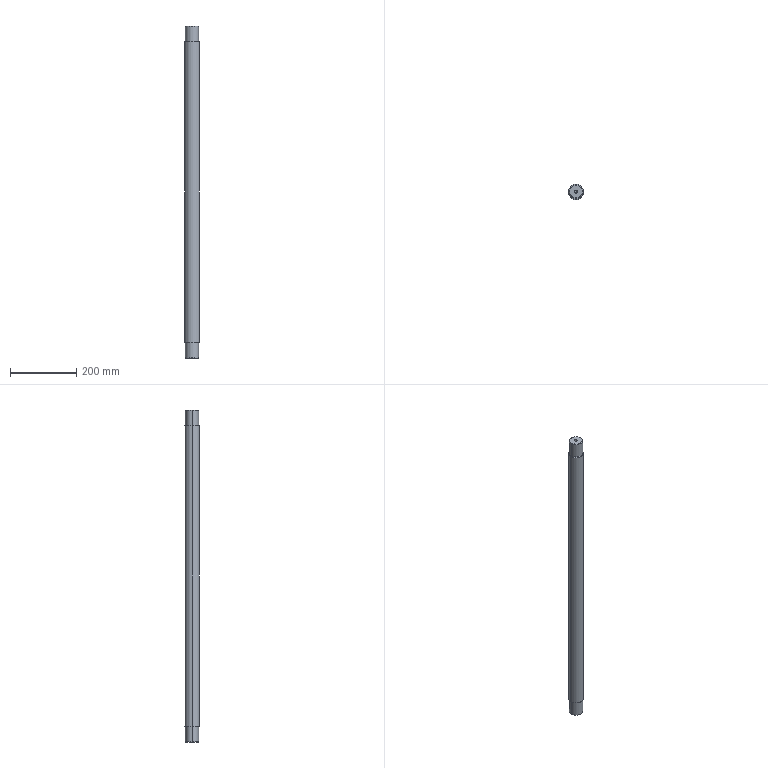Part | SolidWorks | features HoleWzd 2, ICE 2, Chamfer 1, Extrusion 1, Fillet 1 | 1 solid | 26 faces | box 45 x 45 x 1000 mm | volume 1555641 mm3 | cylinder 10 | cone 8 | torus 4 | plane 4 | commonest cylinder face diameters 8.5 x4 40 x4 45 x2
STEP:
#1=CARTESIAN_POINT('',(4.25,0.,-23.2));
#2=VERTEX_POINT('',#1);
#3=CARTESIAN_POINT('',(-4.25,0.,-23.2));
#4=VERTEX_POINT('',#3);
#5=CARTESIAN_POINT('',(0.,0.,-23.2));
#6=DIRECTION('',(0.,0.,-1.));
#7=DIRECTION('',(-1.,0.,0.));
#8=AXIS2_PLACEMENT_3D('',#5,#6,#7);
#9=CIRCLE('',#8,4.25);
#10=EDGE_CURVE('',#2,#4,#9,.T.);
#11=ORIENTED_EDGE('',*,*,#10,.F.);
#12=CARTESIAN_POINT('',(4.25,0.,-47.7));
#13=VERTEX_POINT('',#12);
#14=CARTESIAN_POINT('',(4.25,0.,-47.7));
#15=DIRECTION('',(0.,0.,-1.));
#16=VECTOR('',#15,1000.);
#17=LINE('',#14,#16);
#18=EDGE_CURVE('',#2,#13,#17,.T.);
#19=ORIENTED_EDGE('',*,*,#18,.T.);
#20=CARTESIAN_POINT('',(-4.25,0.,-47.7));
#21=VERTEX_POINT('',#20);
#22=CARTESIAN_POINT('',(0.,0.,-47.7));
#23=DIRECTION('',(0.,0.,-1.));
#24=DIRECTION('',(-1.,0.,0.));
#25=AXIS2_PLACEMENT_3D('',#22,#23,#24);
#26=CIRCLE('',#25,4.25);
#27=EDGE_CURVE('',#13,#21,#26,.T.);
#28=ORIENTED_EDGE('',*,*,#27,.T.);
#29=CARTESIAN_POINT('',(-4.25,0.,-47.7));
#30=DIRECTION('',(0.,0.,-1.));
#31=VECTOR('',#30,1000.);
#32=LINE('',#29,#31);
#33=EDGE_CURVE('',#4,#21,#32,.T.);
#34=ORIENTED_EDGE('',*,*,#33,.F.);
#35=EDGE_LOOP('',(#11,#19,#28,#34));
#36=FACE_OUTER_BOUND('',#35,.T.);
#37=CARTESIAN_POINT('',(0.,0.,-47.7));
#38=DIRECTION('',(0.,0.,-1.));
#39=DIRECTION('',(-1.,0.,0.));
#40=AXIS2_PLACEMENT_3D('',#37,#38,#39);
#41=CYLINDRICAL_SURFACE('',#40,4.25);
#42=ADVANCED_FACE('',(#36),#41,.F.);
#43=CARTESIAN_POINT('',(0.,0.,-20.646));
#44=VERTEX_POINT('',#43);
#45=CARTESIAN_POINT('',(-4.25,0.,-23.2));
#46=DIRECTION('',(-0.8572,0.,-0.515));
#47=VECTOR('',#46,1000.);
#48=LINE('',#45,#47);
#49=EDGE_CURVE('',#44,#4,#48,.T.);
#50=ORIENTED_EDGE('',*,*,#49,.F.);
#51=CARTESIAN_POINT('',(4.25,0.,-23.2));
#52=DIRECTION('',(0.8572,0.,-0.515));
#53=VECTOR('',#52,1000.);
#54=LINE('',#51,#53);
#55=EDGE_CURVE('',#44,#2,#54,.T.);
#56=ORIENTED_EDGE('',*,*,#55,.T.);
#57=ORIENTED_EDGE('',*,*,#10,.T.);
#58=EDGE_LOOP('',(#50,#56,#57));
#59=FACE_OUTER_BOUND('',#58,.T.);
#60=CARTESIAN_POINT('',(0.,0.,-23.2));
#61=DIRECTION('',(0.,0.,-1.));
#62=DIRECTION('',(-1.,0.,0.));
#63=AXIS2_PLACEMENT_3D('',#60,#61,#62);
#64=CONICAL_SURFACE('',#63,4.25,1.03);
#65=ADVANCED_FACE('',(#59),#64,.F.);
#66=CARTESIAN_POINT('',(-4.25,0.,927.8));
#67=VERTEX_POINT('',#66);
#68=CARTESIAN_POINT('',(4.25,0.,927.8));
#69=VERTEX_POINT('',#68);
#70=CARTESIAN_POINT('',(0.,0.,927.8));
#71=DIRECTION('',(0.,0.,1.));
#72=DIRECTION('',(1.,0.,0.));
#73=AXIS2_PLACEMENT_3D('',#70,#71,#72);
#74=CIRCLE('',#73,4.25);
#75=EDGE_CURVE('',#67,#69,#74,.T.);
#76=ORIENTED_EDGE('',*,*,#75,.F.);
#77=CARTESIAN_POINT('',(-4.25,0.,952.3));
#78=VERTEX_POINT('',#77);
#79=CARTESIAN_POINT('',(-4.25,0.,952.3));
#80=DIRECTION('',(0.,0.,1.));
#81=VECTOR('',#80,1000.);
#82=LINE('',#79,#81);
#83=EDGE_CURVE('',#67,#78,#82,.T.);
#84=ORIENTED_EDGE('',*,*,#83,.T.);
#85=CARTESIAN_POINT('',(4.25,0.,952.3));
#86=VERTEX_POINT('',#85);
#87=CARTESIAN_POINT('',(0.,0.,952.3));
#88=DIRECTION('',(0.,0.,1.));
#89=DIRECTION('',(1.,0.,0.));
#90=AXIS2_PLACEMENT_3D('',#87,#88,#89);
#91=CIRCLE('',#90,4.25);
#92=EDGE_CURVE('',#78,#86,#91,.T.);
#93=ORIENTED_EDGE('',*,*,#92,.T.);
#94=CARTESIAN_POINT('',(4.25,0.,952.3));
#95=DIRECTION('',(0.,0.,1.));
#96=VECTOR('',#95,1000.);
#97=LINE('',#94,#96);
#98=EDGE_CURVE('',#69,#86,#97,.T.);
#99=ORIENTED_EDGE('',*,*,#98,.F.);
#100=EDGE_LOOP('',(#76,#84,#93,#99));
#101=FACE_OUTER_BOUND('',#100,.T.);
#102=CARTESIAN_POINT('',(0.,0.,952.3));
#103=DIRECTION('',(0.,0.,1.));
#104=DIRECTION('',(1.,0.,0.));
#105=AXIS2_PLACEMENT_3D('',#102,#103,#104);
#106=CYLINDRICAL_SURFACE('',#105,4.25);
#107=ADVANCED_FACE('',(#101),#106,.F.);
#108=CARTESIAN_POINT('',(0.,0.,925.246));
#109=VERTEX_POINT('',#108);
#110=CARTESIAN_POINT('',(4.25,0.,927.8));
#111=DIRECTION('',(0.8572,0.,0.515));
#112=VECTOR('',#111,1000.);
#113=LINE('',#110,#112);
#114=EDGE_CURVE('',#109,#69,#113,.T.);
#115=ORIENTED_EDGE('',*,*,#114,.F.);
#116=CARTESIAN_POINT('',(-4.25,0.,927.8));
#117=DIRECTION('',(-0.8572,0.,0.515));
#118=VECTOR('',#117,1000.);
#119=LINE('',#116,#118);
#120=EDGE_CURVE('',#109,#67,#119,.T.);
#121=ORIENTED_EDGE('',*,*,#120,.T.);
#122=ORIENTED_EDGE('',*,*,#75,.T.);
#123=EDGE_LOOP('',(#115,#121,#122));
#124=FACE_OUTER_BOUND('',#123,.T.);
#125=CARTESIAN_POINT('',(0.,0.,927.8));
#126=DIRECTION('',(0.,0.,1.));
#127=DIRECTION('',(1.,0.,0.));
#128=AXIS2_PLACEMENT_3D('',#125,#126,#127);
#129=CONICAL_SURFACE('',#128,4.25,1.03);
#130=ADVANCED_FACE('',(#124),#129,.F.);
#131=CARTESIAN_POINT('',(-19.,0.,-47.7));
#132=VERTEX_POINT('',#131);
#133=CARTESIAN_POINT('',(19.,0.,-47.7));
#134=VERTEX_POINT('',#133);
#135=CARTESIAN_POINT('',(0.,0.,-47.7));
#136=DIRECTION('',(0.,0.,-1.));
#137=DIRECTION('',(-1.,0.,0.));
#138=AXIS2_PLACEMENT_3D('',#135,#136,#137);
#139=CIRCLE('',#138,19.);
#140=EDGE_CURVE('',#132,#134,#139,.T.);
#141=ORIENTED_EDGE('',*,*,#140,.F.);
#142=CARTESIAN_POINT('',(-20.,0.,-46.7));
#143=VERTEX_POINT('',#142);
#144=CARTESIAN_POINT('',(-19.,0.,-47.7));
#145=DIRECTION('',(-0.7071,0.,0.7071));
#146=VECTOR('',#145,1000.);
#147=LINE('',#144,#146);
#148=EDGE_CURVE('',#132,#143,#147,.T.);
#149=ORIENTED_EDGE('',*,*,#148,.T.);
#150=CARTESIAN_POINT('',(20.,0.,-46.7));
#151=VERTEX_POINT('',#150);
#152=CARTESIAN_POINT('',(0.,0.,-46.7));
#153=DIRECTION('',(0.,0.,1.));
#154=DIRECTION('',(-1.,0.,0.));
#155=AXIS2_PLACEMENT_3D('',#152,#153,#154);
#156=CIRCLE('',#155,20.);
#157=EDGE_CURVE('',#151,#143,#156,.T.);
#158=ORIENTED_EDGE('',*,*,#157,.F.);
#159=CARTESIAN_POINT('',(19.,0.,-47.7));
#160=DIRECTION('',(0.7071,0.,0.7071));
#161=VECTOR('',#160,1000.);
#162=LINE('',#159,#161);
#163=EDGE_CURVE('',#134,#151,#162,.T.);
#164=ORIENTED_EDGE('',*,*,#163,.F.);
#165=EDGE_LOOP('',(#141,#149,#158,#164));
#166=FACE_OUTER_BOUND('',#165,.T.);
#167=CARTESIAN_POINT('',(0.,0.,-47.7));
#168=DIRECTION('',(0.,0.,1.));
#169=DIRECTION('',(1.,0.,0.));
#170=AXIS2_PLACEMENT_3D('',#167,#168,#169);
#171=CONICAL_SURFACE('',#170,19.,0.7854);
#172=ADVANCED_FACE('',(#166),#171,.T.);
#173=CARTESIAN_POINT('',(19.,0.,952.3));
#174=VERTEX_POINT('',#173);
#175=CARTESIAN_POINT('',(-19.,0.,952.3));
#176=VERTEX_POINT('',#175);
#177=CARTESIAN_POINT('',(0.,0.,952.3));
#178=DIRECTION('',(0.,0.,1.));
#179=DIRECTION('',(1.,0.,0.));
#180=AXIS2_PLACEMENT_3D('',#177,#178,#179);
#181=CIRCLE('',#180,19.);
#182=EDGE_CURVE('',#174,#176,#181,.T.);
#183=ORIENTED_EDGE('',*,*,#182,.F.);
#184=CARTESIAN_POINT('',(20.,0.,951.3));
#185=VERTEX_POINT('',#184);
#186=CARTESIAN_POINT('',(19.,0.,952.3));
#187=DIRECTION('',(0.7071,0.,-0.7071));
#188=VECTOR('',#187,1000.);
#189=LINE('',#186,#188);
#190=EDGE_CURVE('',#174,#185,#189,.T.);
#191=ORIENTED_EDGE('',*,*,#190,.T.);
#192=CARTESIAN_POINT('',(-20.,0.,951.3));
#193=VERTEX_POINT('',#192);
#194=CARTESIAN_POINT('',(0.,0.,951.3));
#195=DIRECTION('',(0.,0.,-1.));
#196=DIRECTION('',(1.,0.,0.));
#197=AXIS2_PLACEMENT_3D('',#194,#195,#196);
#198=CIRCLE('',#197,20.);
#199=EDGE_CURVE('',#193,#185,#198,.T.);
#200=ORIENTED_EDGE('',*,*,#199,.F.);
#201=CARTESIAN_POINT('',(-19.,0.,952.3));
#202=DIRECTION('',(-0.7071,0.,-0.7071));
#203=VECTOR('',#202,1000.);
#204=LINE('',#201,#203);
#205=EDGE_CURVE('',#176,#193,#204,.T.);
#206=ORIENTED_EDGE('',*,*,#205,.F.);
#207=EDGE_LOOP('',(#183,#191,#200,#206));
#208=FACE_OUTER_BOUND('',#207,.T.);
#209=CARTESIAN_POINT('',(0.,0.,952.3));
#210=DIRECTION('',(0.,0.,-1.));
#211=DIRECTION('',(-1.,0.,0.));
#212=AXIS2_PLACEMENT_3D('',#209,#210,#211);
#213=CONICAL_SURFACE('',#212,19.,0.7854);
#214=ADVANCED_FACE('',(#208),#213,.T.);
#215=CARTESIAN_POINT('',(-20.,0.,905.6));
#216=VERTEX_POINT('',#215);
#217=CARTESIAN_POINT('',(20.,0.,905.6));
#218=VERTEX_POINT('',#217);
#219=CARTESIAN_POINT('',(0.,0.,905.6));
#220=DIRECTION('',(0.,0.,1.));
#221=DIRECTION('',(1.,0.,0.));
#222=AXIS2_PLACEMENT_3D('',#219,#220,#221);
#223=CIRCLE('',#222,20.);
#224=EDGE_CURVE('',#216,#218,#223,.T.);
#225=ORIENTED_EDGE('',*,*,#224,.F.);
#226=CARTESIAN_POINT('',(-21.,0.,904.6));
#227=VERTEX_POINT('',#226);
#228=CARTESIAN_POINT('',(-21.,0.,905.6));
#229=DIRECTION('',(0.,1.,0.));
#230=DIRECTION('',(-1.,0.,0.));
#231=AXIS2_PLACEMENT_3D('',#228,#229,#230);
#232=CIRCLE('',#231,1.);
#233=EDGE_CURVE('',#216,#227,#232,.T.);
#234=ORIENTED_EDGE('',*,*,#233,.T.);
#235=CARTESIAN_POINT('',(21.,0.,904.6));
#236=VERTEX_POINT('',#235);
#237=CARTESIAN_POINT('',(0.,0.,904.6));
#238=DIRECTION('',(0.,0.,-1.));
#239=DIRECTION('',(1.,0.,0.));
#240=AXIS2_PLACEMENT_3D('',#237,#238,#239);
#241=CIRCLE('',#240,21.);
#242=EDGE_CURVE('',#236,#227,#241,.T.);
#243=ORIENTED_EDGE('',*,*,#242,.F.);
#244=CARTESIAN_POINT('',(21.,0.,905.6));
#245=DIRECTION('',(0.,-1.,0.));
#246=DIRECTION('',(0.,0.,-1.));
#247=AXIS2_PLACEMENT_3D('',#244,#245,#246);
#248=CIRCLE('',#247,1.);
#249=EDGE_CURVE('',#218,#236,#248,.T.);
#250=ORIENTED_EDGE('',*,*,#249,.F.);
#251=EDGE_LOOP('',(#225,#234,#243,#250));
#252=FACE_OUTER_BOUND('',#251,.T.);
#253=CARTESIAN_POINT('',(0.,0.,905.6));
#254=DIRECTION('',(0.,0.,1.));
#255=DIRECTION('',(1.,0.,0.));
#256=AXIS2_PLACEMENT_3D('',#253,#254,#255);
#257=TOROIDAL_SURFACE('',#256,21.,1.);
#258=ADVANCED_FACE('',(#252),#257,.F.);
#259=CARTESIAN_POINT('',(-21.,0.,0.));
#260=VERTEX_POINT('',#259);
#261=CARTESIAN_POINT('',(21.,0.,0.));
#262=VERTEX_POINT('',#261);
#263=CARTESIAN_POINT('',(0.,0.,0.));
#264=DIRECTION('',(0.,0.,1.));
#265=DIRECTION('',(1.,0.,0.));
#266=AXIS2_PLACEMENT_3D('',#263,#264,#265);
#267=CIRCLE('',#266,21.);
#268=EDGE_CURVE('',#260,#262,#267,.T.);
#269=ORIENTED_EDGE('',*,*,#268,.F.);
#270=CARTESIAN_POINT('',(-20.,0.,-1.));
#271=VERTEX_POINT('',#270);
#272=CARTESIAN_POINT('',(-21.,0.,-1.));
#273=DIRECTION('',(0.,1.,0.));
#274=DIRECTION('',(-1.,0.,0.));
#275=AXIS2_PLACEMENT_3D('',#272,#273,#274);
#276=CIRCLE('',#275,1.);
#277=EDGE_CURVE('',#260,#271,#276,.T.);
#278=ORIENTED_EDGE('',*,*,#277,.T.);
#279=CARTESIAN_POINT('',(20.,0.,-1.));
#280=VERTEX_POINT('',#279);
#281=CARTESIAN_POINT('',(0.,0.,-1.));
#282=DIRECTION('',(0.,0.,-1.));
#283=DIRECTION('',(1.,0.,0.));
#284=AXIS2_PLACEMENT_3D('',#281,#282,#283);
#285=CIRCLE('',#284,20.);
#286=EDGE_CURVE('',#280,#271,#285,.T.);
#287=ORIENTED_EDGE('',*,*,#286,.F.);
#288=CARTESIAN_POINT('',(21.,0.,-1.));
#289=DIRECTION('',(0.,-1.,0.));
#290=DIRECTION('',(0.,0.,-1.));
#291=AXIS2_PLACEMENT_3D('',#288,#289,#290);
#292=CIRCLE('',#291,1.);
#293=EDGE_CURVE('',#262,#280,#292,.T.);
#294=ORIENTED_EDGE('',*,*,#293,.F.);
#295=EDGE_LOOP('',(#269,#278,#287,#294));
#296=FACE_OUTER_BOUND('',#295,.T.);
#297=CARTESIAN_POINT('',(0.,0.,-1.));
#298=DIRECTION('',(0.,0.,1.));
#299=DIRECTION('',(1.,0.,0.));
#300=AXIS2_PLACEMENT_3D('',#297,#298,#299);
#301=TOROIDAL_SURFACE('',#300,21.,1.);
#302=ADVANCED_FACE('',(#296),#301,.F.);
#303=ORIENTED_EDGE('',*,*,#157,.T.);
#304=CARTESIAN_POINT('',(-20.,0.,-47.7));
#305=DIRECTION('',(0.,0.,1.));
#306=VECTOR('',#305,1000.);
#307=LINE('',#304,#306);
#308=EDGE_CURVE('',#143,#271,#307,.T.);
#309=ORIENTED_EDGE('',*,*,#308,.T.);
#310=CARTESIAN_POINT('',(0.,0.,-1.));
#311=DIRECTION('',(0.,0.,-1.));
#312=DIRECTION('',(1.,0.,0.));
#313=AXIS2_PLACEMENT_3D('',#310,#311,#312);
#314=CIRCLE('',#313,20.);
#315=EDGE_CURVE('',#271,#280,#314,.T.);
#316=ORIENTED_EDGE('',*,*,#315,.T.);
#317=CARTESIAN_POINT('',(20.,0.,-47.7));
#318=DIRECTION('',(0.,0.,1.));
#319=VECTOR('',#318,1000.);
#320=LINE('',#317,#319);
#321=EDGE_CURVE('',#151,#280,#320,.T.);
#322=ORIENTED_EDGE('',*,*,#321,.F.);
#323=EDGE_LOOP('',(#303,#309,#316,#322));
#324=FACE_OUTER_BOUND('',#323,.T.);
#325=CARTESIAN_POINT('',(0.,0.,-47.7));
#326=DIRECTION('',(0.,0.,1.));
#327=DIRECTION('',(1.,0.,0.));
#328=AXIS2_PLACEMENT_3D('',#325,#326,#327);
#329=CYLINDRICAL_SURFACE('',#328,20.);
#330=ADVANCED_FACE('',(#324),#329,.T.);
#331=ORIENTED_EDGE('',*,*,#199,.T.);
#332=CARTESIAN_POINT('',(20.,0.,952.3));
#333=DIRECTION('',(0.,0.,-1.));
#334=VECTOR('',#333,1000.);
#335=LINE('',#332,#334);
#336=EDGE_CURVE('',#185,#218,#335,.T.);
#337=ORIENTED_EDGE('',*,*,#336,.T.);
#338=CARTESIAN_POINT('',(0.,0.,905.6));
#339=DIRECTION('',(0.,0.,1.));
#340=DIRECTION('',(1.,0.,0.));
#341=AXIS2_PLACEMENT_3D('',#338,#339,#340);
#342=CIRCLE('',#341,20.);
#343=EDGE_CURVE('',#218,#216,#342,.T.);
#344=ORIENTED_EDGE('',*,*,#343,.T.);
#345=CARTESIAN_POINT('',(-20.,0.,952.3));
#346=DIRECTION('',(0.,0.,-1.));
#347=VECTOR('',#346,1000.);
#348=LINE('',#345,#347);
#349=EDGE_CURVE('',#193,#216,#348,.T.);
#350=ORIENTED_EDGE('',*,*,#349,.F.);
#351=EDGE_LOOP('',(#331,#337,#344,#350));
#352=FACE_OUTER_BOUND('',#351,.T.);
#353=CARTESIAN_POINT('',(0.,0.,952.3));
#354=DIRECTION('',(0.,0.,-1.));
#355=DIRECTION('',(-1.,0.,0.));
#356=AXIS2_PLACEMENT_3D('',#353,#354,#355);
#357=CYLINDRICAL_SURFACE('',#356,20.);
#358=ADVANCED_FACE('',(#352),#357,.T.);
#359=CARTESIAN_POINT('',(22.5,0.,904.6));
#360=VERTEX_POINT('',#359);
#361=CARTESIAN_POINT('',(-22.5,0.,904.6));
#362=VERTEX_POINT('',#361);
#363=CARTESIAN_POINT('',(0.,0.,904.6));
#364=DIRECTION('',(0.,0.,1.));
#365=DIRECTION('',(1.,0.,0.));
#366=AXIS2_PLACEMENT_3D('',#363,#364,#365);
#367=CIRCLE('',#366,22.5);
#368=EDGE_CURVE('',#360,#362,#367,.T.);
#369=ORIENTED_EDGE('',*,*,#368,.F.);
#370=CARTESIAN_POINT('',(22.5,0.,0.));
#371=VERTEX_POINT('',#370);
#372=CARTESIAN_POINT('',(22.5,0.,904.6));
#373=DIRECTION('',(0.,0.,-1.));
#374=VECTOR('',#373,1000.);
#375=LINE('',#372,#374);
#376=EDGE_CURVE('',#360,#371,#375,.T.);
#377=ORIENTED_EDGE('',*,*,#376,.T.);
#378=CARTESIAN_POINT('',(-22.5,0.,0.));
#379=VERTEX_POINT('',#378);
#380=CARTESIAN_POINT('',(0.,0.,0.));
#381=DIRECTION('',(0.,0.,1.));
#382=DIRECTION('',(1.,0.,0.));
#383=AXIS2_PLACEMENT_3D('',#380,#381,#382);
#384=CIRCLE('',#383,22.5);
#385=EDGE_CURVE('',#371,#379,#384,.T.);
#386=ORIENTED_EDGE('',*,*,#385,.T.);
#387=CARTESIAN_POINT('',(-22.5,0.,904.6));
#388=DIRECTION('',(0.,0.,-1.));
#389=VECTOR('',#388,1000.);
#390=LINE('',#387,#389);
#391=EDGE_CURVE('',#362,#379,#390,.T.);
#392=ORIENTED_EDGE('',*,*,#391,.F.);
#393=EDGE_LOOP('',(#369,#377,#386,#392));
#394=FACE_OUTER_BOUND('',#393,.T.);
#395=CARTESIAN_POINT('',(0.,0.,904.6));
#396=DIRECTION('',(0.,0.,-1.));
#397=DIRECTION('',(-1.,0.,0.));
#398=AXIS2_PLACEMENT_3D('',#395,#396,#397);
#399=CYLINDRICAL_SURFACE('',#398,22.5);
#400=ADVANCED_FACE('',(#394),#399,.T.);
#401=ORIENTED_EDGE('',*,*,#376,.F.);
#402=CARTESIAN_POINT('',(0.,0.,904.6));
#403=DIRECTION('',(0.,0.,1.));
#404=DIRECTION('',(1.,0.,0.));
#405=AXIS2_PLACEMENT_3D('',#402,#403,#404);
#406=CIRCLE('',#405,22.5);
#407=EDGE_CURVE('',#362,#360,#406,.T.);
#408=ORIENTED_EDGE('',*,*,#407,.F.);
#409=ORIENTED_EDGE('',*,*,#391,.T.);
#410=CARTESIAN_POINT('',(0.,0.,0.));
#411=DIRECTION('',(0.,0.,1.));
#412=DIRECTION('',(1.,0.,0.));
#413=AXIS2_PLACEMENT_3D('',#410,#411,#412);
#414=CIRCLE('',#413,22.5);
#415=EDGE_CURVE('',#379,#371,#414,.T.);
#416=ORIENTED_EDGE('',*,*,#415,.T.);
#417=EDGE_LOOP('',(#401,#408,#409,#416));
#418=FACE_OUTER_BOUND('',#417,.T.);
#419=CARTESIAN_POINT('',(0.,0.,904.6));
#420=DIRECTION('',(0.,0.,-1.));
#421=DIRECTION('',(-1.,0.,0.));
#422=AXIS2_PLACEMENT_3D('',#419,#420,#421);
#423=CYLINDRICAL_SURFACE('',#422,22.5);
#424=ADVANCED_FACE('',(#418),#423,.T.);
#425=ORIENTED_EDGE('',*,*,#242,.T.);
#426=CARTESIAN_POINT('',(0.,0.,904.6));
#427=DIRECTION('',(0.,0.,-1.));
#428=DIRECTION('',(1.,0.,0.));
#429=AXIS2_PLACEMENT_3D('',#426,#427,#428);
#430=CIRCLE('',#429,21.);
#431=EDGE_CURVE('',#227,#236,#430,.T.);
#432=ORIENTED_EDGE('',*,*,#431,.T.);
#433=EDGE_LOOP('',(#425,#432));
#434=FACE_BOUND('',#433,.T.);
#435=ORIENTED_EDGE('',*,*,#407,.T.);
#436=ORIENTED_EDGE('',*,*,#368,.T.);
#437=EDGE_LOOP('',(#435,#436));
#438=FACE_OUTER_BOUND('',#437,.T.);
#439=CARTESIAN_POINT('',(0.,0.,904.6));
#440=DIRECTION('',(0.,0.,1.));
#441=DIRECTION('',(1.,0.,0.));
#442=AXIS2_PLACEMENT_3D('',#439,#440,#441);
#443=PLANE('',#442);
#444=ADVANCED_FACE('',(#434,#438),#443,.T.);
#445=CARTESIAN_POINT('',(0.,0.,0.));
#446=DIRECTION('',(0.,0.,1.));
#447=DIRECTION('',(1.,0.,0.));
#448=AXIS2_PLACEMENT_3D('',#445,#446,#447);
#449=CIRCLE('',#448,21.);
#450=EDGE_CURVE('',#262,#260,#449,.T.);
#451=ORIENTED_EDGE('',*,*,#450,.T.);
#452=ORIENTED_EDGE('',*,*,#268,.T.);
#453=EDGE_LOOP('',(#451,#452));
#454=FACE_BOUND('',#453,.T.);
#455=ORIENTED_EDGE('',*,*,#415,.F.);
#456=ORIENTED_EDGE('',*,*,#385,.F.);
#457=EDGE_LOOP('',(#455,#456));
#458=FACE_OUTER_BOUND('',#457,.T.);
#459=CARTESIAN_POINT('',(0.,0.,0.));
#460=DIRECTION('',(0.,0.,1.));
#461=DIRECTION('',(1.,0.,0.));
#462=AXIS2_PLACEMENT_3D('',#459,#460,#461);
#463=PLANE('',#462);
#464=ADVANCED_FACE('',(#454,#458),#463,.F.);
#465=ORIENTED_EDGE('',*,*,#336,.F.);
#466=CARTESIAN_POINT('',(0.,0.,951.3));
#467=DIRECTION('',(0.,0.,-1.));
#468=DIRECTION('',(1.,0.,0.));
#469=AXIS2_PLACEMENT_3D('',#466,#467,#468);
#470=CIRCLE('',#469,20.);
#471=EDGE_CURVE('',#185,#193,#470,.T.);
#472=ORIENTED_EDGE('',*,*,#471,.T.);
#473=ORIENTED_EDGE('',*,*,#349,.T.);
#474=ORIENTED_EDGE('',*,*,#224,.T.);
#475=EDGE_LOOP('',(#465,#472,#473,#474));
#476=FACE_OUTER_BOUND('',#475,.T.);
#477=CARTESIAN_POINT('',(0.,0.,952.3));
#478=DIRECTION('',(0.,0.,-1.));
#479=DIRECTION('',(-1.,0.,0.));
#480=AXIS2_PLACEMENT_3D('',#477,#478,#479);
#481=CYLINDRICAL_SURFACE('',#480,20.);
#482=ADVANCED_FACE('',(#476),#481,.T.);
#483=CARTESIAN_POINT('',(0.,0.,952.3));
#484=DIRECTION('',(0.,0.,1.));
#485=DIRECTION('',(1.,0.,0.));
#486=AXIS2_PLACEMENT_3D('',#483,#484,#485);
#487=CIRCLE('',#486,4.25);
#488=EDGE_CURVE('',#86,#78,#487,.T.);
#489=ORIENTED_EDGE('',*,*,#488,.F.);
#490=ORIENTED_EDGE('',*,*,#92,.F.);
#491=EDGE_LOOP('',(#489,#490));
#492=FACE_BOUND('',#491,.T.);
#493=CARTESIAN_POINT('',(0.,0.,952.3));
#494=DIRECTION('',(0.,0.,1.));
#495=DIRECTION('',(1.,0.,0.));
#496=AXIS2_PLACEMENT_3D('',#493,#494,#495);
#497=CIRCLE('',#496,19.);
#498=EDGE_CURVE('',#176,#174,#497,.T.);
#499=ORIENTED_EDGE('',*,*,#498,.T.);
#500=ORIENTED_EDGE('',*,*,#182,.T.);
#501=EDGE_LOOP('',(#499,#500));
#502=FACE_OUTER_BOUND('',#501,.T.);
#503=CARTESIAN_POINT('',(0.,0.,952.3));
#504=DIRECTION('',(0.,0.,1.));
#505=DIRECTION('',(1.,0.,0.));
#506=AXIS2_PLACEMENT_3D('',#503,#504,#505);
#507=PLANE('',#506);
#508=ADVANCED_FACE('',(#492,#502),#507,.T.);
#509=ORIENTED_EDGE('',*,*,#308,.F.);
#510=CARTESIAN_POINT('',(0.,0.,-46.7));
#511=DIRECTION('',(0.,0.,1.));
#512=DIRECTION('',(-1.,0.,0.));
#513=AXIS2_PLACEMENT_3D('',#510,#511,#512);
#514=CIRCLE('',#513,20.);
#515=EDGE_CURVE('',#143,#151,#514,.T.);
#516=ORIENTED_EDGE('',*,*,#515,.T.);
#517=ORIENTED_EDGE('',*,*,#321,.T.);
#518=ORIENTED_EDGE('',*,*,#286,.T.);
#519=EDGE_LOOP('',(#509,#516,#517,#518));
#520=FACE_OUTER_BOUND('',#519,.T.);
#521=CARTESIAN_POINT('',(0.,0.,-47.7));
#522=DIRECTION('',(0.,0.,1.));
#523=DIRECTION('',(1.,0.,0.));
#524=AXIS2_PLACEMENT_3D('',#521,#522,#523);
#525=CYLINDRICAL_SURFACE('',#524,20.);
#526=ADVANCED_FACE('',(#520),#525,.T.);
#527=CARTESIAN_POINT('',(0.,0.,-47.7));
#528=DIRECTION('',(0.,0.,-1.));
#529=DIRECTION('',(-1.,0.,0.));
#530=AXIS2_PLACEMENT_3D('',#527,#528,#529);
#531=CIRCLE('',#530,4.25);
#532=EDGE_CURVE('',#21,#13,#531,.T.);
#533=ORIENTED_EDGE('',*,*,#532,.F.);
#534=ORIENTED_EDGE('',*,*,#27,.F.);
#535=EDGE_LOOP('',(#533,#534));
#536=FACE_BOUND('',#535,.T.);
#537=CARTESIAN_POINT('',(0.,0.,-47.7));
#538=DIRECTION('',(0.,0.,-1.));
#539=DIRECTION('',(-1.,0.,0.));
#540=AXIS2_PLACEMENT_3D('',#537,#538,#539);
#541=CIRCLE('',#540,19.);
#542=EDGE_CURVE('',#134,#132,#541,.T.);
#543=ORIENTED_EDGE('',*,*,#542,.T.);
#544=ORIENTED_EDGE('',*,*,#140,.T.);
#545=EDGE_LOOP('',(#543,#544));
#546=FACE_OUTER_BOUND('',#545,.T.);
#547=CARTESIAN_POINT('',(0.,0.,-47.7));
#548=DIRECTION('',(0.,0.,-1.));
#549=DIRECTION('',(-1.,0.,0.));
#550=AXIS2_PLACEMENT_3D('',#547,#548,#549);
#551=PLANE('',#550);
#552=ADVANCED_FACE('',(#536,#546),#551,.T.);
#553=ORIENTED_EDGE('',*,*,#277,.F.);
#554=ORIENTED_EDGE('',*,*,#450,.F.);
#555=ORIENTED_EDGE('',*,*,#293,.T.);
#556=ORIENTED_EDGE('',*,*,#315,.F.);
#557=EDGE_LOOP('',(#553,#554,#555,#556));
#558=FACE_OUTER_BOUND('',#557,.T.);
#559=CARTESIAN_POINT('',(0.,0.,-1.));
#560=DIRECTION('',(0.,0.,1.));
#561=DIRECTION('',(1.,0.,0.));
#562=AXIS2_PLACEMENT_3D('',#559,#560,#561);
#563=TOROIDAL_SURFACE('',#562,21.,1.);
#564=ADVANCED_FACE('',(#558),#563,.F.);
#565=ORIENTED_EDGE('',*,*,#233,.F.);
#566=ORIENTED_EDGE('',*,*,#343,.F.);
#567=ORIENTED_EDGE('',*,*,#249,.T.);
#568=ORIENTED_EDGE('',*,*,#431,.F.);
#569=EDGE_LOOP('',(#565,#566,#567,#568));
#570=FACE_OUTER_BOUND('',#569,.T.);
#571=CARTESIAN_POINT('',(0.,0.,905.6));
#572=DIRECTION('',(0.,0.,1.));
#573=DIRECTION('',(1.,0.,0.));
#574=AXIS2_PLACEMENT_3D('',#571,#572,#573);
#575=TOROIDAL_SURFACE('',#574,21.,1.);
#576=ADVANCED_FACE('',(#570),#575,.F.);
#577=ORIENTED_EDGE('',*,*,#190,.F.);
#578=ORIENTED_EDGE('',*,*,#498,.F.);
#579=ORIENTED_EDGE('',*,*,#205,.T.);
#580=ORIENTED_EDGE('',*,*,#471,.F.);
#581=EDGE_LOOP('',(#577,#578,#579,#580));
#582=FACE_OUTER_BOUND('',#581,.T.);
#583=CARTESIAN_POINT('',(0.,0.,952.3));
#584=DIRECTION('',(0.,0.,-1.));
#585=DIRECTION('',(-1.,0.,0.));
#586=AXIS2_PLACEMENT_3D('',#583,#584,#585);
#587=CONICAL_SURFACE('',#586,19.,0.7854);
#588=ADVANCED_FACE('',(#582),#587,.T.);
#589=ORIENTED_EDGE('',*,*,#148,.F.);
#590=ORIENTED_EDGE('',*,*,#542,.F.);
#591=ORIENTED_EDGE('',*,*,#163,.T.);
#592=ORIENTED_EDGE('',*,*,#515,.F.);
#593=EDGE_LOOP('',(#589,#590,#591,#592));
#594=FACE_OUTER_BOUND('',#593,.T.);
#595=CARTESIAN_POINT('',(0.,0.,-47.7));
#596=DIRECTION('',(0.,0.,1.));
#597=DIRECTION('',(1.,0.,0.));
#598=AXIS2_PLACEMENT_3D('',#595,#596,#597);
#599=CONICAL_SURFACE('',#598,19.,0.7854);
#600=ADVANCED_FACE('',(#594),#599,.T.);
#601=ORIENTED_EDGE('',*,*,#120,.F.);
#602=ORIENTED_EDGE('',*,*,#114,.T.);
#603=CARTESIAN_POINT('',(0.,0.,927.8));
#604=DIRECTION('',(0.,0.,1.));
#605=DIRECTION('',(1.,0.,0.));
#606=AXIS2_PLACEMENT_3D('',#603,#604,#605);
#607=CIRCLE('',#606,4.25);
#608=EDGE_CURVE('',#69,#67,#607,.T.);
#609=ORIENTED_EDGE('',*,*,#608,.T.);
#610=EDGE_LOOP('',(#601,#602,#609));
#611=FACE_OUTER_BOUND('',#610,.T.);
#612=CARTESIAN_POINT('',(0.,0.,927.8));
#613=DIRECTION('',(0.,0.,1.));
#614=DIRECTION('',(1.,0.,0.));
#615=AXIS2_PLACEMENT_3D('',#612,#613,#614);
#616=CONICAL_SURFACE('',#615,4.25,1.03);
#617=ADVANCED_FACE('',(#611),#616,.F.);
#618=ORIENTED_EDGE('',*,*,#83,.F.);
#619=ORIENTED_EDGE('',*,*,#608,.F.);
#620=ORIENTED_EDGE('',*,*,#98,.T.);
#621=ORIENTED_EDGE('',*,*,#488,.T.);
#622=EDGE_LOOP('',(#618,#619,#620,#621));
#623=FACE_OUTER_BOUND('',#622,.T.);
#624=CARTESIAN_POINT('',(0.,0.,952.3));
#625=DIRECTION('',(0.,0.,1.));
#626=DIRECTION('',(1.,0.,0.));
#627=AXIS2_PLACEMENT_3D('',#624,#625,#626);
#628=CYLINDRICAL_SURFACE('',#627,4.25);
#629=ADVANCED_FACE('',(#623),#628,.F.);
#630=ORIENTED_EDGE('',*,*,#55,.F.);
#631=ORIENTED_EDGE('',*,*,#49,.T.);
#632=CARTESIAN_POINT('',(0.,0.,-23.2));
#633=DIRECTION('',(0.,0.,-1.));
#634=DIRECTION('',(-1.,0.,0.));
#635=AXIS2_PLACEMENT_3D('',#632,#633,#634);
#636=CIRCLE('',#635,4.25);
#637=EDGE_CURVE('',#4,#2,#636,.T.);
#638=ORIENTED_EDGE('',*,*,#637,.T.);
#639=EDGE_LOOP('',(#630,#631,#638));
#640=FACE_OUTER_BOUND('',#639,.T.);
#641=CARTESIAN_POINT('',(0.,0.,-23.2));
#642=DIRECTION('',(0.,0.,-1.));
#643=DIRECTION('',(-1.,0.,0.));
#644=AXIS2_PLACEMENT_3D('',#641,#642,#643);
#645=CONICAL_SURFACE('',#644,4.25,1.03);
#646=ADVANCED_FACE('',(#640),#645,.F.);
#647=ORIENTED_EDGE('',*,*,#18,.F.);
#648=ORIENTED_EDGE('',*,*,#637,.F.);
#649=ORIENTED_EDGE('',*,*,#33,.T.);
#650=ORIENTED_EDGE('',*,*,#532,.T.);
#651=EDGE_LOOP('',(#647,#648,#649,#650));
#652=FACE_OUTER_BOUND('',#651,.T.);
#653=CARTESIAN_POINT('',(0.,0.,-47.7));
#654=DIRECTION('',(0.,0.,-1.));
#655=DIRECTION('',(-1.,0.,0.));
#656=AXIS2_PLACEMENT_3D('',#653,#654,#655);
#657=CYLINDRICAL_SURFACE('',#656,4.25);
#658=ADVANCED_FACE('',(#652),#657,.F.);
#659=CLOSED_SHELL('',(#42,#65,#107,#130,#172,#214,#258,#302,#330,#358,#400,#424,#444,#464,#482,#508,#526,#552,#564,#576,#588,#600,#617,#629,#646,#658));
#660=MANIFOLD_SOLID_BREP('',#659);
#661=CARTESIAN_POINT('',(0.,0.,0.));
#662=DIRECTION('',(0.,0.,1.));
#663=DIRECTION('',(1.,0.,0.));
#664=AXIS2_PLACEMENT_3D('',#661,#662,#663);
#665=(LENGTH_UNIT()NAMED_UNIT(*)SI_UNIT(.MILLI.,.METRE.));
#666=UNCERTAINTY_MEASURE_WITH_UNIT(LENGTH_MEASURE(0.00001),#665,'','');
#667=(NAMED_UNIT(*)PLANE_ANGLE_UNIT()SI_UNIT($,.RADIAN.));
#668=(NAMED_UNIT(*)SI_UNIT($,.STERADIAN.)SOLID_ANGLE_UNIT());
#669=(GEOMETRIC_REPRESENTATION_CONTEXT(3)GLOBAL_UNCERTAINTY_ASSIGNED_CONTEXT((#666))GLOBAL_UNIT_ASSIGNED_CONTEXT((#665,#667,#668))REPRESENTATION_CONTEXT('',''));
#670=ADVANCED_BREP_SHAPE_REPRESENTATION('',(#660,#664),#669);